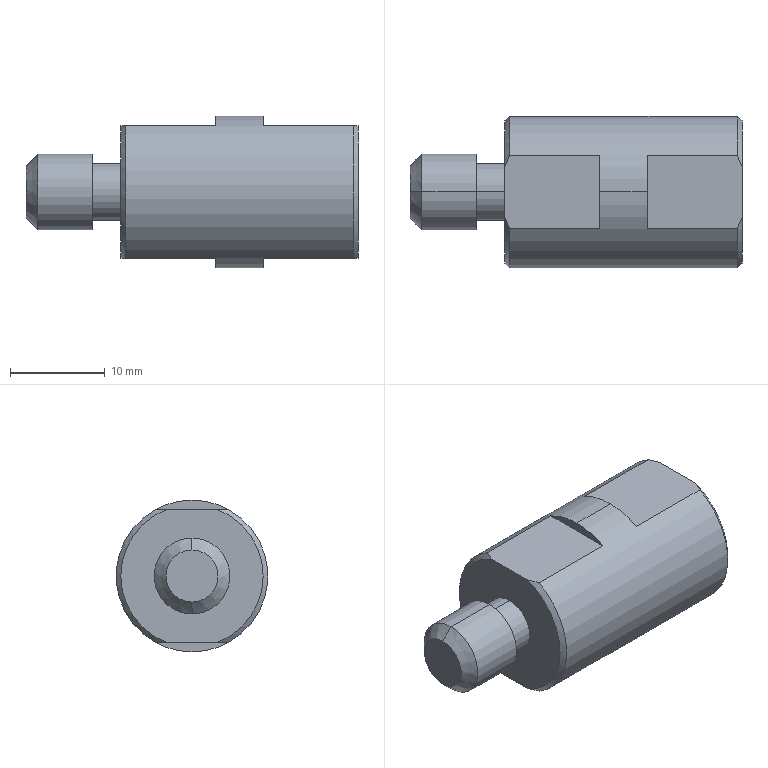Part | STEP file | PSSAGD16-27-F10-M8-N8-WSC0-X0-4 | 1 solid | 32 faces | box 35 x 16 x 16 mm | volume 4383 mm3 | plane 12 | cylinder 10 | cone 10 | commonest cylinder face diameters 8 x4 6 x2 6.647 x2 16 x2
STEP:
#1=CARTESIAN_POINT('',(4.919,0.,3.324));
#2=VERTEX_POINT('',#1);
#3=CARTESIAN_POINT('',(4.919,0.,-3.324));
#4=VERTEX_POINT('',#3);
#5=CARTESIAN_POINT('',(4.919,0.,0.));
#6=DIRECTION('',(1.,0.,0.));
#7=DIRECTION('',(0.,0.,-1.));
#8=AXIS2_PLACEMENT_3D('',#5,#6,#7);
#9=CIRCLE('',#8,3.324);
#10=EDGE_CURVE('',#2,#4,#9,.T.);
#11=ORIENTED_EDGE('',*,*,#10,.F.);
#12=CARTESIAN_POINT('',(16.591,0.,3.324));
#13=VERTEX_POINT('',#12);
#14=CARTESIAN_POINT('',(27.,0.,3.324));
#15=DIRECTION('',(1.,0.,0.));
#16=VECTOR('',#15,1000.);
#17=LINE('',#14,#16);
#18=EDGE_CURVE('',#2,#13,#17,.T.);
#19=ORIENTED_EDGE('',*,*,#18,.T.);
#20=CARTESIAN_POINT('',(16.591,0.,-3.323));
#21=VERTEX_POINT('',#20);
#22=CARTESIAN_POINT('',(16.591,0.,0.));
#23=DIRECTION('',(-1.,0.,0.));
#24=DIRECTION('',(0.,0.,-1.));
#25=AXIS2_PLACEMENT_3D('',#22,#23,#24);
#26=CIRCLE('',#25,3.324);
#27=EDGE_CURVE('',#21,#13,#26,.T.);
#28=ORIENTED_EDGE('',*,*,#27,.F.);
#29=CARTESIAN_POINT('',(27.,0.,-3.324));
#30=DIRECTION('',(1.,0.,0.));
#31=VECTOR('',#30,1000.);
#32=LINE('',#29,#31);
#33=EDGE_CURVE('',#4,#21,#32,.T.);
#34=ORIENTED_EDGE('',*,*,#33,.F.);
#35=EDGE_LOOP('',(#11,#19,#28,#34));
#36=FACE_OUTER_BOUND('',#35,.T.);
#37=CARTESIAN_POINT('',(27.,0.,0.));
#38=DIRECTION('',(1.,0.,0.));
#39=DIRECTION('',(0.,0.,-1.));
#40=AXIS2_PLACEMENT_3D('',#37,#38,#39);
#41=CYLINDRICAL_SURFACE('',#40,3.324);
#42=ADVANCED_FACE('',(#36),#41,.F.);
#43=CARTESIAN_POINT('',(3.,0.,0.));
#44=VERTEX_POINT('',#43);
#45=CARTESIAN_POINT('',(3.,0.,0.));
#46=DIRECTION('',(0.5,0.,-0.866));
#47=VECTOR('',#46,1000.);
#48=LINE('',#45,#47);
#49=EDGE_CURVE('',#44,#4,#48,.T.);
#50=ORIENTED_EDGE('',*,*,#49,.F.);
#51=CARTESIAN_POINT('',(3.,0.,0.));
#52=DIRECTION('',(0.5,0.,0.866));
#53=VECTOR('',#52,1000.);
#54=LINE('',#51,#53);
#55=EDGE_CURVE('',#44,#2,#54,.T.);
#56=ORIENTED_EDGE('',*,*,#55,.T.);
#57=ORIENTED_EDGE('',*,*,#10,.T.);
#58=EDGE_LOOP('',(#50,#56,#57));
#59=FACE_OUTER_BOUND('',#58,.T.);
#60=CARTESIAN_POINT('',(1003.,0.,0.));
#61=DIRECTION('',(1.,0.,0.));
#62=DIRECTION('',(0.,0.,-1.));
#63=AXIS2_PLACEMENT_3D('',#60,#61,#62);
#64=CONICAL_SURFACE('',#63,1732.051,1.047);
#65=ADVANCED_FACE('',(#59),#64,.F.);
#66=ORIENTED_EDGE('',*,*,#27,.T.);
#67=CARTESIAN_POINT('',(17.267,0.,4.));
#68=VERTEX_POINT('',#67);
#69=CARTESIAN_POINT('',(17.267,0.,4.));
#70=DIRECTION('',(0.7071,0.,0.7071));
#71=VECTOR('',#70,1000.);
#72=LINE('',#69,#71);
#73=EDGE_CURVE('',#13,#68,#72,.T.);
#74=ORIENTED_EDGE('',*,*,#73,.T.);
#75=CARTESIAN_POINT('',(17.267,0.,-4.));
#76=VERTEX_POINT('',#75);
#77=CARTESIAN_POINT('',(17.267,0.,0.));
#78=DIRECTION('',(-1.,0.,0.));
#79=DIRECTION('',(0.,0.,1.));
#80=AXIS2_PLACEMENT_3D('',#77,#78,#79);
#81=CIRCLE('',#80,4.);
#82=EDGE_CURVE('',#76,#68,#81,.T.);
#83=ORIENTED_EDGE('',*,*,#82,.F.);
#84=CARTESIAN_POINT('',(17.267,0.,-4.));
#85=DIRECTION('',(0.7071,0.,-0.7071));
#86=VECTOR('',#85,1000.);
#87=LINE('',#84,#86);
#88=EDGE_CURVE('',#21,#76,#87,.T.);
#89=ORIENTED_EDGE('',*,*,#88,.F.);
#90=EDGE_LOOP('',(#66,#74,#83,#89));
#91=FACE_OUTER_BOUND('',#90,.T.);
#92=CARTESIAN_POINT('',(17.267,0.,0.));
#93=DIRECTION('',(1.,0.,0.));
#94=DIRECTION('',(0.,0.,-1.));
#95=AXIS2_PLACEMENT_3D('',#92,#93,#94);
#96=CONICAL_SURFACE('',#95,4.,0.7854);
#97=ADVANCED_FACE('',(#91),#96,.F.);
#98=CARTESIAN_POINT('',(25.,0.,-4.));
#99=VERTEX_POINT('',#98);
#100=CARTESIAN_POINT('',(25.,0.,4.));
#101=VERTEX_POINT('',#100);
#102=CARTESIAN_POINT('',(25.,0.,0.));
#103=DIRECTION('',(-1.,0.,0.));
#104=DIRECTION('',(0.,0.,1.));
#105=AXIS2_PLACEMENT_3D('',#102,#103,#104);
#106=CIRCLE('',#105,4.);
#107=EDGE_CURVE('',#99,#101,#106,.T.);
#108=ORIENTED_EDGE('',*,*,#107,.F.);
#109=CARTESIAN_POINT('',(16.5,0.,-4.));
#110=DIRECTION('',(-1.,0.,0.));
#111=VECTOR('',#110,1000.);
#112=LINE('',#109,#111);
#113=EDGE_CURVE('',#99,#76,#112,.T.);
#114=ORIENTED_EDGE('',*,*,#113,.T.);
#115=ORIENTED_EDGE('',*,*,#82,.T.);
#116=CARTESIAN_POINT('',(16.5,0.,4.));
#117=DIRECTION('',(-1.,0.,0.));
#118=VECTOR('',#117,1000.);
#119=LINE('',#116,#118);
#120=EDGE_CURVE('',#101,#68,#119,.T.);
#121=ORIENTED_EDGE('',*,*,#120,.F.);
#122=EDGE_LOOP('',(#108,#114,#115,#121));
#123=FACE_OUTER_BOUND('',#122,.T.);
#124=CARTESIAN_POINT('',(16.5,0.,0.));
#125=DIRECTION('',(-1.,0.,0.));
#126=DIRECTION('',(0.,0.,1.));
#127=AXIS2_PLACEMENT_3D('',#124,#125,#126);
#128=CYLINDRICAL_SURFACE('',#127,4.);
#129=ADVANCED_FACE('',(#123),#128,.F.);
#130=CARTESIAN_POINT('',(-3.,0.,-3.));
#131=VERTEX_POINT('',#130);
#132=CARTESIAN_POINT('',(-3.,0.,3.));
#133=VERTEX_POINT('',#132);
#134=CARTESIAN_POINT('',(-3.,0.,0.));
#135=DIRECTION('',(1.,0.,0.));
#136=DIRECTION('',(0.,0.,-1.));
#137=AXIS2_PLACEMENT_3D('',#134,#135,#136);
#138=CIRCLE('',#137,3.);
#139=EDGE_CURVE('',#131,#133,#138,.T.);
#140=ORIENTED_EDGE('',*,*,#139,.T.);
#141=CARTESIAN_POINT('',(0.,0.,3.));
#142=VERTEX_POINT('',#141);
#143=CARTESIAN_POINT('',(27.,0.,3.));
#144=DIRECTION('',(1.,0.,0.));
#145=VECTOR('',#144,1000.);
#146=LINE('',#143,#145);
#147=EDGE_CURVE('',#133,#142,#146,.T.);
#148=ORIENTED_EDGE('',*,*,#147,.T.);
#149=CARTESIAN_POINT('',(0.,0.,-3.));
#150=VERTEX_POINT('',#149);
#151=CARTESIAN_POINT('',(0.,0.,0.));
#152=DIRECTION('',(1.,0.,0.));
#153=DIRECTION('',(0.,0.,-1.));
#154=AXIS2_PLACEMENT_3D('',#151,#152,#153);
#155=CIRCLE('',#154,3.);
#156=EDGE_CURVE('',#150,#142,#155,.T.);
#157=ORIENTED_EDGE('',*,*,#156,.F.);
#158=CARTESIAN_POINT('',(27.,0.,-3.));
#159=DIRECTION('',(1.,0.,0.));
#160=VECTOR('',#159,1000.);
#161=LINE('',#158,#160);
#162=EDGE_CURVE('',#131,#150,#161,.T.);
#163=ORIENTED_EDGE('',*,*,#162,.F.);
#164=EDGE_LOOP('',(#140,#148,#157,#163));
#165=FACE_OUTER_BOUND('',#164,.T.);
#166=CARTESIAN_POINT('',(27.,0.,0.));
#167=DIRECTION('',(1.,0.,0.));
#168=DIRECTION('',(0.,0.,-1.));
#169=AXIS2_PLACEMENT_3D('',#166,#167,#168);
#170=CYLINDRICAL_SURFACE('',#169,3.);
#171=ADVANCED_FACE('',(#165),#170,.T.);
#172=CARTESIAN_POINT('',(-8.75,0.,-4.));
#173=VERTEX_POINT('',#172);
#174=CARTESIAN_POINT('',(-8.75,0.,4.));
#175=VERTEX_POINT('',#174);
#176=CARTESIAN_POINT('',(-8.75,0.,0.));
#177=DIRECTION('',(1.,0.,0.));
#178=DIRECTION('',(0.,0.,-1.));
#179=AXIS2_PLACEMENT_3D('',#176,#177,#178);
#180=CIRCLE('',#179,4.);
#181=EDGE_CURVE('',#173,#175,#180,.T.);
#182=ORIENTED_EDGE('',*,*,#181,.T.);
#183=CARTESIAN_POINT('',(-3.,0.,4.));
#184=VERTEX_POINT('',#183);
#185=CARTESIAN_POINT('',(27.,0.,4.));
#186=DIRECTION('',(1.,0.,0.));
#187=VECTOR('',#186,1000.);
#188=LINE('',#185,#187);
#189=EDGE_CURVE('',#175,#184,#188,.T.);
#190=ORIENTED_EDGE('',*,*,#189,.T.);
#191=CARTESIAN_POINT('',(-3.,0.,-4.));
#192=VERTEX_POINT('',#191);
#193=CARTESIAN_POINT('',(-3.,0.,0.));
#194=DIRECTION('',(1.,0.,0.));
#195=DIRECTION('',(0.,0.,-1.));
#196=AXIS2_PLACEMENT_3D('',#193,#194,#195);
#197=CIRCLE('',#196,4.);
#198=EDGE_CURVE('',#192,#184,#197,.T.);
#199=ORIENTED_EDGE('',*,*,#198,.F.);
#200=CARTESIAN_POINT('',(27.,0.,-4.));
#201=DIRECTION('',(1.,0.,0.));
#202=VECTOR('',#201,1000.);
#203=LINE('',#200,#202);
#204=EDGE_CURVE('',#173,#192,#203,.T.);
#205=ORIENTED_EDGE('',*,*,#204,.F.);
#206=EDGE_LOOP('',(#182,#190,#199,#205));
#207=FACE_OUTER_BOUND('',#206,.T.);
#208=CARTESIAN_POINT('',(27.,0.,0.));
#209=DIRECTION('',(1.,0.,0.));
#210=DIRECTION('',(0.,0.,-1.));
#211=AXIS2_PLACEMENT_3D('',#208,#209,#210);
#212=CYLINDRICAL_SURFACE('',#211,4.);
#213=ADVANCED_FACE('',(#207),#212,.T.);
#214=CARTESIAN_POINT('',(-10.,0.,-2.75));
#215=VERTEX_POINT('',#214);
#216=CARTESIAN_POINT('',(-10.,0.,2.75));
#217=VERTEX_POINT('',#216);
#218=CARTESIAN_POINT('',(-10.,0.,0.));
#219=DIRECTION('',(1.,0.,0.));
#220=DIRECTION('',(0.,0.,-1.));
#221=AXIS2_PLACEMENT_3D('',#218,#219,#220);
#222=CIRCLE('',#221,2.75);
#223=EDGE_CURVE('',#215,#217,#222,.T.);
#224=ORIENTED_EDGE('',*,*,#223,.T.);
#225=CARTESIAN_POINT('',(-10.,0.,2.75));
#226=DIRECTION('',(0.7071,0.,0.7071));
#227=VECTOR('',#226,1000.);
#228=LINE('',#225,#227);
#229=EDGE_CURVE('',#217,#175,#228,.T.);
#230=ORIENTED_EDGE('',*,*,#229,.T.);
#231=ORIENTED_EDGE('',*,*,#181,.F.);
#232=CARTESIAN_POINT('',(-10.,0.,-2.75));
#233=DIRECTION('',(0.7071,0.,-0.7071));
#234=VECTOR('',#233,1000.);
#235=LINE('',#232,#234);
#236=EDGE_CURVE('',#215,#173,#235,.T.);
#237=ORIENTED_EDGE('',*,*,#236,.F.);
#238=EDGE_LOOP('',(#224,#230,#231,#237));
#239=FACE_OUTER_BOUND('',#238,.T.);
#240=CARTESIAN_POINT('',(-10.,0.,0.));
#241=DIRECTION('',(1.,0.,0.));
#242=DIRECTION('',(0.,0.,-1.));
#243=AXIS2_PLACEMENT_3D('',#240,#241,#242);
#244=CONICAL_SURFACE('',#243,2.75,0.7854);
#245=ADVANCED_FACE('',(#239),#244,.T.);
#246=CARTESIAN_POINT('',(10.,3.873,7.));
#247=VERTEX_POINT('',#246);
#248=CARTESIAN_POINT('',(10.,0.,8.));
#249=VERTEX_POINT('',#248);
#250=CARTESIAN_POINT('',(10.,0.,0.));
#251=DIRECTION('',(1.,0.,0.));
#252=DIRECTION('',(0.,0.,-1.));
#253=AXIS2_PLACEMENT_3D('',#250,#251,#252);
#254=CIRCLE('',#253,8.);
#255=EDGE_CURVE('',#247,#249,#254,.T.);
#256=ORIENTED_EDGE('',*,*,#255,.T.);
#257=CARTESIAN_POINT('',(15.,0.,8.));
#258=VERTEX_POINT('',#257);
#259=CARTESIAN_POINT('',(27.,0.,8.));
#260=DIRECTION('',(1.,0.,0.));
#261=VECTOR('',#260,1000.);
#262=LINE('',#259,#261);
#263=EDGE_CURVE('',#249,#258,#262,.T.);
#264=ORIENTED_EDGE('',*,*,#263,.T.);
#265=CARTESIAN_POINT('',(15.,3.873,7.));
#266=VERTEX_POINT('',#265);
#267=CARTESIAN_POINT('',(15.,0.,0.));
#268=DIRECTION('',(1.,0.,0.));
#269=DIRECTION('',(0.,0.,-1.));
#270=AXIS2_PLACEMENT_3D('',#267,#268,#269);
#271=CIRCLE('',#270,8.);
#272=EDGE_CURVE('',#266,#258,#271,.T.);
#273=ORIENTED_EDGE('',*,*,#272,.F.);
#274=CARTESIAN_POINT('',(24.5,3.873,7.));
#275=VERTEX_POINT('',#274);
#276=CARTESIAN_POINT('',(25.,3.873,7.));
#277=DIRECTION('',(-1.,0.,0.));
#278=VECTOR('',#277,1000.);
#279=LINE('',#276,#278);
#280=EDGE_CURVE('',#275,#266,#279,.T.);
#281=ORIENTED_EDGE('',*,*,#280,.F.);
#282=CARTESIAN_POINT('',(24.5,3.873,-7.));
#283=VERTEX_POINT('',#282);
#284=CARTESIAN_POINT('',(24.5,0.,0.));
#285=DIRECTION('',(1.,0.,0.));
#286=DIRECTION('',(0.,0.,-1.));
#287=AXIS2_PLACEMENT_3D('',#284,#285,#286);
#288=CIRCLE('',#287,8.);
#289=EDGE_CURVE('',#283,#275,#288,.T.);
#290=ORIENTED_EDGE('',*,*,#289,.F.);
#291=CARTESIAN_POINT('',(15.,3.873,-7.));
#292=VERTEX_POINT('',#291);
#293=CARTESIAN_POINT('',(25.,3.873,-7.));
#294=DIRECTION('',(1.,0.,0.));
#295=VECTOR('',#294,1000.);
#296=LINE('',#293,#295);
#297=EDGE_CURVE('',#292,#283,#296,.T.);
#298=ORIENTED_EDGE('',*,*,#297,.F.);
#299=CARTESIAN_POINT('',(15.,0.,-8.));
#300=VERTEX_POINT('',#299);
#301=CARTESIAN_POINT('',(15.,0.,0.));
#302=DIRECTION('',(1.,0.,0.));
#303=DIRECTION('',(0.,0.,-1.));
#304=AXIS2_PLACEMENT_3D('',#301,#302,#303);
#305=CIRCLE('',#304,8.);
#306=EDGE_CURVE('',#300,#292,#305,.T.);
#307=ORIENTED_EDGE('',*,*,#306,.F.);
#308=CARTESIAN_POINT('',(10.,0.,-8.));
#309=VERTEX_POINT('',#308);
#310=CARTESIAN_POINT('',(27.,0.,-8.));
#311=DIRECTION('',(1.,0.,0.));
#312=VECTOR('',#311,1000.);
#313=LINE('',#310,#312);
#314=EDGE_CURVE('',#309,#300,#313,.T.);
#315=ORIENTED_EDGE('',*,*,#314,.F.);
#316=CARTESIAN_POINT('',(10.,3.873,-7.));
#317=VERTEX_POINT('',#316);
#318=CARTESIAN_POINT('',(10.,0.,0.));
#319=DIRECTION('',(1.,0.,0.));
#320=DIRECTION('',(0.,0.,-1.));
#321=AXIS2_PLACEMENT_3D('',#318,#319,#320);
#322=CIRCLE('',#321,8.);
#323=EDGE_CURVE('',#309,#317,#322,.T.);
#324=ORIENTED_EDGE('',*,*,#323,.T.);
#325=CARTESIAN_POINT('',(0.5,3.873,-7.));
#326=VERTEX_POINT('',#325);
#327=CARTESIAN_POINT('',(27.,3.873,-7.));
#328=DIRECTION('',(-1.,0.,0.));
#329=VECTOR('',#328,1000.);
#330=LINE('',#327,#329);
#331=EDGE_CURVE('',#317,#326,#330,.T.);
#332=ORIENTED_EDGE('',*,*,#331,.T.);
#333=CARTESIAN_POINT('',(0.5,3.873,7.));
#334=VERTEX_POINT('',#333);
#335=CARTESIAN_POINT('',(0.5,0.,0.));
#336=DIRECTION('',(1.,0.,0.));
#337=DIRECTION('',(0.,0.,-1.));
#338=AXIS2_PLACEMENT_3D('',#335,#336,#337);
#339=CIRCLE('',#338,8.);
#340=EDGE_CURVE('',#326,#334,#339,.T.);
#341=ORIENTED_EDGE('',*,*,#340,.T.);
#342=CARTESIAN_POINT('',(27.,3.873,7.));
#343=DIRECTION('',(1.,0.,0.));
#344=VECTOR('',#343,1000.);
#345=LINE('',#342,#344);
#346=EDGE_CURVE('',#334,#247,#345,.T.);
#347=ORIENTED_EDGE('',*,*,#346,.T.);
#348=EDGE_LOOP('',(#256,#264,#273,#281,#290,#298,#307,#315,#324,#332,#341,#347));
#349=FACE_OUTER_BOUND('',#348,.T.);
#350=CARTESIAN_POINT('',(27.,0.,0.));
#351=DIRECTION('',(1.,0.,0.));
#352=DIRECTION('',(0.,0.,-1.));
#353=AXIS2_PLACEMENT_3D('',#350,#351,#352);
#354=CYLINDRICAL_SURFACE('',#353,8.);
#355=ADVANCED_FACE('',(#349),#354,.T.);
#356=ORIENTED_EDGE('',*,*,#263,.F.);
#357=CARTESIAN_POINT('',(10.,-3.873,7.));
#358=VERTEX_POINT('',#357);
#359=CARTESIAN_POINT('',(10.,0.,0.));
#360=DIRECTION('',(1.,0.,0.));
#361=DIRECTION('',(0.,0.,-1.));
#362=AXIS2_PLACEMENT_3D('',#359,#360,#361);
#363=CIRCLE('',#362,8.);
#364=EDGE_CURVE('',#249,#358,#363,.T.);
#365=ORIENTED_EDGE('',*,*,#364,.T.);
#366=CARTESIAN_POINT('',(0.5,-3.873,7.));
#367=VERTEX_POINT('',#366);
#368=CARTESIAN_POINT('',(27.,-3.873,7.));
#369=DIRECTION('',(-1.,0.,0.));
#370=VECTOR('',#369,1000.);
#371=LINE('',#368,#370);
#372=EDGE_CURVE('',#358,#367,#371,.T.);
#373=ORIENTED_EDGE('',*,*,#372,.T.);
#374=CARTESIAN_POINT('',(0.5,-3.873,-7.));
#375=VERTEX_POINT('',#374);
#376=CARTESIAN_POINT('',(0.5,0.,0.));
#377=DIRECTION('',(1.,0.,0.));
#378=DIRECTION('',(0.,0.,-1.));
#379=AXIS2_PLACEMENT_3D('',#376,#377,#378);
#380=CIRCLE('',#379,8.);
#381=EDGE_CURVE('',#367,#375,#380,.T.);
#382=ORIENTED_EDGE('',*,*,#381,.T.);
#383=CARTESIAN_POINT('',(10.,-3.873,-7.));
#384=VERTEX_POINT('',#383);
#385=CARTESIAN_POINT('',(27.,-3.873,-7.));
#386=DIRECTION('',(1.,0.,0.));
#387=VECTOR('',#386,1000.);
#388=LINE('',#385,#387);
#389=EDGE_CURVE('',#375,#384,#388,.T.);
#390=ORIENTED_EDGE('',*,*,#389,.T.);
#391=CARTESIAN_POINT('',(10.,0.,0.));
#392=DIRECTION('',(1.,0.,0.));
#393=DIRECTION('',(0.,0.,-1.));
#394=AXIS2_PLACEMENT_3D('',#391,#392,#393);
#395=CIRCLE('',#394,8.);
#396=EDGE_CURVE('',#384,#309,#395,.T.);
#397=ORIENTED_EDGE('',*,*,#396,.T.);
#398=ORIENTED_EDGE('',*,*,#314,.T.);
#399=CARTESIAN_POINT('',(15.,-3.873,-7.));
#400=VERTEX_POINT('',#399);
#401=CARTESIAN_POINT('',(15.,0.,0.));
#402=DIRECTION('',(1.,0.,0.));
#403=DIRECTION('',(0.,0.,-1.));
#404=AXIS2_PLACEMENT_3D('',#401,#402,#403);
#405=CIRCLE('',#404,8.);
#406=EDGE_CURVE('',#400,#300,#405,.T.);
#407=ORIENTED_EDGE('',*,*,#406,.F.);
#408=CARTESIAN_POINT('',(24.5,-3.873,-7.));
#409=VERTEX_POINT('',#408);
#410=CARTESIAN_POINT('',(25.,-3.873,-7.));
#411=DIRECTION('',(-1.,0.,0.));
#412=VECTOR('',#411,1000.);
#413=LINE('',#410,#412);
#414=EDGE_CURVE('',#409,#400,#413,.T.);
#415=ORIENTED_EDGE('',*,*,#414,.F.);
#416=CARTESIAN_POINT('',(24.5,-3.873,7.));
#417=VERTEX_POINT('',#416);
#418=CARTESIAN_POINT('',(24.5,0.,0.));
#419=DIRECTION('',(1.,0.,0.));
#420=DIRECTION('',(0.,0.,-1.));
#421=AXIS2_PLACEMENT_3D('',#418,#419,#420);
#422=CIRCLE('',#421,8.);
#423=EDGE_CURVE('',#417,#409,#422,.T.);
#424=ORIENTED_EDGE('',*,*,#423,.F.);
#425=CARTESIAN_POINT('',(15.,-3.873,7.));
#426=VERTEX_POINT('',#425);
#427=CARTESIAN_POINT('',(25.,-3.873,7.));
#428=DIRECTION('',(1.,0.,0.));
#429=VECTOR('',#428,1000.);
#430=LINE('',#427,#429);
#431=EDGE_CURVE('',#426,#417,#430,.T.);
#432=ORIENTED_EDGE('',*,*,#431,.F.);
#433=CARTESIAN_POINT('',(15.,0.,0.));
#434=DIRECTION('',(1.,0.,0.));
#435=DIRECTION('',(0.,0.,-1.));
#436=AXIS2_PLACEMENT_3D('',#433,#434,#435);
#437=CIRCLE('',#436,8.);
#438=EDGE_CURVE('',#258,#426,#437,.T.);
#439=ORIENTED_EDGE('',*,*,#438,.F.);
#440=EDGE_LOOP('',(#356,#365,#373,#382,#390,#397,#398,#407,#415,#424,#432,#439));
#441=FACE_OUTER_BOUND('',#440,.T.);
#442=CARTESIAN_POINT('',(27.,0.,0.));
#443=DIRECTION('',(1.,0.,0.));
#444=DIRECTION('',(0.,0.,-1.));
#445=AXIS2_PLACEMENT_3D('',#442,#443,#444);
#446=CYLINDRICAL_SURFACE('',#445,8.);
#447=ADVANCED_FACE('',(#441),#446,.T.);
#448=CARTESIAN_POINT('',(25.,-2.693,-7.));
#449=VERTEX_POINT('',#448);
#450=CARTESIAN_POINT('',(25.,-2.693,-7.));
#451=CARTESIAN_POINT('',(24.856,-3.095,-7.));
#452=CARTESIAN_POINT('',(24.687,-3.487,-7.));
#453=CARTESIAN_POINT('',(24.5,-3.873,-7.));
#454=B_SPLINE_CURVE_WITH_KNOTS('',3,(#450,#451,#452,#453),.UNSPECIFIED.,.F.,.F.,(4,4),(0.006725,0.007986),.UNSPECIFIED.);
#455=EDGE_CURVE('',#449,#409,#454,.T.);
#456=ORIENTED_EDGE('',*,*,#455,.F.);
#457=CARTESIAN_POINT('',(25.,-2.693,7.));
#458=VERTEX_POINT('',#457);
#459=CARTESIAN_POINT('',(25.,0.,0.));
#460=DIRECTION('',(1.,0.,0.));
#461=DIRECTION('',(0.,0.,-1.));
#462=AXIS2_PLACEMENT_3D('',#459,#460,#461);
#463=CIRCLE('',#462,7.5);
#464=EDGE_CURVE('',#458,#449,#463,.T.);
#465=ORIENTED_EDGE('',*,*,#464,.F.);
#466=CARTESIAN_POINT('',(24.5,-3.873,7.));
#467=CARTESIAN_POINT('',(24.688,-3.486,7.));
#468=CARTESIAN_POINT('',(24.856,-3.093,7.));
#469=CARTESIAN_POINT('',(25.,-2.693,7.));
#470=B_SPLINE_CURVE_WITH_KNOTS('',3,(#466,#467,#468,#469),.UNSPECIFIED.,.F.,.F.,(4,4),(0.000001583,0.001274),.UNSPECIFIED.);
#471=EDGE_CURVE('',#417,#458,#470,.T.);
#472=ORIENTED_EDGE('',*,*,#471,.F.);
#473=ORIENTED_EDGE('',*,*,#423,.T.);
#474=EDGE_LOOP('',(#456,#465,#472,#473));
#475=FACE_OUTER_BOUND('',#474,.T.);
#476=CARTESIAN_POINT('',(24.5,0.,0.));
#477=DIRECTION('',(-1.,0.,0.));
#478=DIRECTION('',(0.,0.,1.));
#479=AXIS2_PLACEMENT_3D('',#476,#477,#478);
#480=CONICAL_SURFACE('',#479,8.,0.7854);
#481=ADVANCED_FACE('',(#475),#480,.T.);
#482=CARTESIAN_POINT('',(25.,2.693,7.));
#483=VERTEX_POINT('',#482);
#484=CARTESIAN_POINT('',(25.,2.693,7.));
#485=CARTESIAN_POINT('',(24.856,3.095,7.));
#486=CARTESIAN_POINT('',(24.687,3.487,7.));
#487=CARTESIAN_POINT('',(24.5,3.873,7.));
#488=B_SPLINE_CURVE_WITH_KNOTS('',3,(#484,#485,#486,#487),.UNSPECIFIED.,.F.,.F.,(4,4),(0.006725,0.007986),.UNSPECIFIED.);
#489=EDGE_CURVE('',#483,#275,#488,.T.);
#490=ORIENTED_EDGE('',*,*,#489,.F.);
#491=CARTESIAN_POINT('',(25.,2.693,-7.));
#492=VERTEX_POINT('',#491);
#493=CARTESIAN_POINT('',(25.,0.,0.));
#494=DIRECTION('',(1.,0.,0.));
#495=DIRECTION('',(0.,0.,-1.));
#496=AXIS2_PLACEMENT_3D('',#493,#494,#495);
#497=CIRCLE('',#496,7.5);
#498=EDGE_CURVE('',#492,#483,#497,.T.);
#499=ORIENTED_EDGE('',*,*,#498,.F.);
#500=CARTESIAN_POINT('',(24.5,3.873,-7.));
#501=CARTESIAN_POINT('',(24.688,3.486,-7.));
#502=CARTESIAN_POINT('',(24.856,3.093,-7.));
#503=CARTESIAN_POINT('',(25.,2.693,-7.));
#504=B_SPLINE_CURVE_WITH_KNOTS('',3,(#500,#501,#502,#503),.UNSPECIFIED.,.F.,.F.,(4,4),(0.000001583,0.001274),.UNSPECIFIED.);
#505=EDGE_CURVE('',#283,#492,#504,.T.);
#506=ORIENTED_EDGE('',*,*,#505,.F.);
#507=ORIENTED_EDGE('',*,*,#289,.T.);
#508=EDGE_LOOP('',(#490,#499,#506,#507));
#509=FACE_OUTER_BOUND('',#508,.T.);
#510=CARTESIAN_POINT('',(24.5,0.,0.));
#511=DIRECTION('',(-1.,0.,0.));
#512=DIRECTION('',(0.,0.,1.));
#513=AXIS2_PLACEMENT_3D('',#510,#511,#512);
#514=CONICAL_SURFACE('',#513,8.,0.7854);
#515=ADVANCED_FACE('',(#509),#514,.T.);
#516=CARTESIAN_POINT('',(25.,0.,0.));
#517=DIRECTION('',(-1.,0.,0.));
#518=DIRECTION('',(0.,0.,1.));
#519=AXIS2_PLACEMENT_3D('',#516,#517,#518);
#520=CIRCLE('',#519,4.);
#521=EDGE_CURVE('',#101,#99,#520,.T.);
#522=ORIENTED_EDGE('',*,*,#521,.T.);
#523=ORIENTED_EDGE('',*,*,#107,.T.);
#524=EDGE_LOOP('',(#522,#523));
#525=FACE_BOUND('',#524,.T.);
#526=CARTESIAN_POINT('',(25.,7.5,-7.));
#527=DIRECTION('',(0.,-1.,0.));
#528=VECTOR('',#527,1000.);
#529=LINE('',#526,#528);
#530=EDGE_CURVE('',#492,#449,#529,.T.);
#531=ORIENTED_EDGE('',*,*,#530,.F.);
#532=ORIENTED_EDGE('',*,*,#498,.T.);
#533=CARTESIAN_POINT('',(25.,7.5,7.));
#534=DIRECTION('',(0.,1.,0.));
#535=VECTOR('',#534,1000.);
#536=LINE('',#533,#535);
#537=EDGE_CURVE('',#458,#483,#536,.T.);
#538=ORIENTED_EDGE('',*,*,#537,.F.);
#539=ORIENTED_EDGE('',*,*,#464,.T.);
#540=EDGE_LOOP('',(#531,#532,#538,#539));
#541=FACE_OUTER_BOUND('',#540,.T.);
#542=CARTESIAN_POINT('',(25.,7.5,0.));
#543=DIRECTION('',(-1.,0.,0.));
#544=DIRECTION('',(0.,0.,1.));
#545=AXIS2_PLACEMENT_3D('',#542,#543,#544);
#546=PLANE('',#545);
#547=ADVANCED_FACE('',(#525,#541),#546,.F.);
#548=CARTESIAN_POINT('',(0.,-2.693,7.));
#549=VERTEX_POINT('',#548);
#550=CARTESIAN_POINT('',(0.,-2.693,-7.));
#551=VERTEX_POINT('',#550);
#552=CARTESIAN_POINT('',(0.,0.,0.));
#553=DIRECTION('',(1.,0.,0.));
#554=DIRECTION('',(0.,0.,-1.));
#555=AXIS2_PLACEMENT_3D('',#552,#553,#554);
#556=CIRCLE('',#555,7.5);
#557=EDGE_CURVE('',#549,#551,#556,.T.);
#558=ORIENTED_EDGE('',*,*,#557,.T.);
#559=CARTESIAN_POINT('',(0.,-2.693,-7.));
#560=CARTESIAN_POINT('',(0.1444,-3.095,-7.));
#561=CARTESIAN_POINT('',(0.3133,-3.487,-7.));
#562=CARTESIAN_POINT('',(0.5,-3.873,-7.));
#563=B_SPLINE_CURVE_WITH_KNOTS('',3,(#559,#560,#561,#562),.UNSPECIFIED.,.F.,.F.,(4,4),(0.006725,0.007986),.UNSPECIFIED.);
#564=EDGE_CURVE('',#551,#375,#563,.T.);
#565=ORIENTED_EDGE('',*,*,#564,.T.);
#566=ORIENTED_EDGE('',*,*,#381,.F.);
#567=CARTESIAN_POINT('',(0.5,-3.873,7.));
#568=CARTESIAN_POINT('',(0.3124,-3.486,7.));
#569=CARTESIAN_POINT('',(0.1437,-3.093,7.));
#570=CARTESIAN_POINT('',(0.,-2.693,7.));
#571=B_SPLINE_CURVE_WITH_KNOTS('',3,(#567,#568,#569,#570),.UNSPECIFIED.,.F.,.F.,(4,4),(0.000001583,0.001274),.UNSPECIFIED.);
#572=EDGE_CURVE('',#367,#549,#571,.T.);
#573=ORIENTED_EDGE('',*,*,#572,.T.);
#574=EDGE_LOOP('',(#558,#565,#566,#573));
#575=FACE_OUTER_BOUND('',#574,.T.);
#576=CARTESIAN_POINT('',(0.,0.,0.));
#577=DIRECTION('',(1.,0.,0.));
#578=DIRECTION('',(0.,0.,-1.));
#579=AXIS2_PLACEMENT_3D('',#576,#577,#578);
#580=CONICAL_SURFACE('',#579,7.5,0.7854);
#581=ADVANCED_FACE('',(#575),#580,.T.);
#582=ORIENTED_EDGE('',*,*,#223,.F.);
#583=CARTESIAN_POINT('',(-10.,0.,0.));
#584=DIRECTION('',(1.,0.,0.));
#585=DIRECTION('',(0.,0.,-1.));
#586=AXIS2_PLACEMENT_3D('',#583,#584,#585);
#587=CIRCLE('',#586,2.75);
#588=EDGE_CURVE('',#217,#215,#587,.T.);
#589=ORIENTED_EDGE('',*,*,#588,.F.);
#590=EDGE_LOOP('',(#582,#589));
#591=FACE_OUTER_BOUND('',#590,.T.);
#592=CARTESIAN_POINT('',(-10.,0.,0.));
#593=DIRECTION('',(1.,0.,0.));
#594=DIRECTION('',(0.,0.,-1.));
#595=AXIS2_PLACEMENT_3D('',#592,#593,#594);
#596=PLANE('',#595);
#597=ADVANCED_FACE('',(#591),#596,.F.);
#598=ORIENTED_EDGE('',*,*,#229,.F.);
#599=ORIENTED_EDGE('',*,*,#588,.T.);
#600=ORIENTED_EDGE('',*,*,#236,.T.);
#601=CARTESIAN_POINT('',(-8.75,0.,0.));
#602=DIRECTION('',(1.,0.,0.));
#603=DIRECTION('',(0.,0.,-1.));
#604=AXIS2_PLACEMENT_3D('',#601,#602,#603);
#605=CIRCLE('',#604,4.);
#606=EDGE_CURVE('',#175,#173,#605,.T.);
#607=ORIENTED_EDGE('',*,*,#606,.F.);
#608=EDGE_LOOP('',(#598,#599,#600,#607));
#609=FACE_OUTER_BOUND('',#608,.T.);
#610=CARTESIAN_POINT('',(-10.,0.,0.));
#611=DIRECTION('',(1.,0.,0.));
#612=DIRECTION('',(0.,0.,-1.));
#613=AXIS2_PLACEMENT_3D('',#610,#611,#612);
#614=CONICAL_SURFACE('',#613,2.75,0.7854);
#615=ADVANCED_FACE('',(#609),#614,.T.);
#616=ORIENTED_EDGE('',*,*,#189,.F.);
#617=ORIENTED_EDGE('',*,*,#606,.T.);
#618=ORIENTED_EDGE('',*,*,#204,.T.);
#619=CARTESIAN_POINT('',(-3.,0.,0.));
#620=DIRECTION('',(1.,0.,0.));
#621=DIRECTION('',(0.,0.,-1.));
#622=AXIS2_PLACEMENT_3D('',#619,#620,#621);
#623=CIRCLE('',#622,4.);
#624=EDGE_CURVE('',#184,#192,#623,.T.);
#625=ORIENTED_EDGE('',*,*,#624,.F.);
#626=EDGE_LOOP('',(#616,#617,#618,#625));
#627=FACE_OUTER_BOUND('',#626,.T.);
#628=CARTESIAN_POINT('',(27.,0.,0.));
#629=DIRECTION('',(1.,0.,0.));
#630=DIRECTION('',(0.,0.,-1.));
#631=AXIS2_PLACEMENT_3D('',#628,#629,#630);
#632=CYLINDRICAL_SURFACE('',#631,4.);
#633=ADVANCED_FACE('',(#627),#632,.T.);
#634=ORIENTED_EDGE('',*,*,#139,.F.);
#635=CARTESIAN_POINT('',(-3.,0.,0.));
#636=DIRECTION('',(1.,0.,0.));
#637=DIRECTION('',(0.,0.,-1.));
#638=AXIS2_PLACEMENT_3D('',#635,#636,#637);
#639=CIRCLE('',#638,3.);
#640=EDGE_CURVE('',#133,#131,#639,.T.);
#641=ORIENTED_EDGE('',*,*,#640,.F.);
#642=EDGE_LOOP('',(#634,#641));
#643=FACE_BOUND('',#642,.T.);
#644=ORIENTED_EDGE('',*,*,#198,.T.);
#645=ORIENTED_EDGE('',*,*,#624,.T.);
#646=EDGE_LOOP('',(#644,#645));
#647=FACE_OUTER_BOUND('',#646,.T.);
#648=CARTESIAN_POINT('',(-3.,4.,0.));
#649=DIRECTION('',(-1.,0.,0.));
#650=DIRECTION('',(0.,0.,1.));
#651=AXIS2_PLACEMENT_3D('',#648,#649,#650);
#652=PLANE('',#651);
#653=ADVANCED_FACE('',(#643,#647),#652,.F.);
#654=ORIENTED_EDGE('',*,*,#147,.F.);
#655=ORIENTED_EDGE('',*,*,#640,.T.);
#656=ORIENTED_EDGE('',*,*,#162,.T.);
#657=CARTESIAN_POINT('',(0.,0.,0.));
#658=DIRECTION('',(1.,0.,0.));
#659=DIRECTION('',(0.,0.,-1.));
#660=AXIS2_PLACEMENT_3D('',#657,#658,#659);
#661=CIRCLE('',#660,3.);
#662=EDGE_CURVE('',#142,#150,#661,.T.);
#663=ORIENTED_EDGE('',*,*,#662,.F.);
#664=EDGE_LOOP('',(#654,#655,#656,#663));
#665=FACE_OUTER_BOUND('',#664,.T.);
#666=CARTESIAN_POINT('',(27.,0.,0.));
#667=DIRECTION('',(1.,0.,0.));
#668=DIRECTION('',(0.,0.,-1.));
#669=AXIS2_PLACEMENT_3D('',#666,#667,#668);
#670=CYLINDRICAL_SURFACE('',#669,3.);
#671=ADVANCED_FACE('',(#665),#670,.T.);
#672=CARTESIAN_POINT('',(0.,2.693,-7.));
#673=VERTEX_POINT('',#672);
#674=CARTESIAN_POINT('',(0.,2.693,7.));
#675=VERTEX_POINT('',#674);
#676=CARTESIAN_POINT('',(0.,0.,0.));
#677=DIRECTION('',(1.,0.,0.));
#678=DIRECTION('',(0.,0.,-1.));
#679=AXIS2_PLACEMENT_3D('',#676,#677,#678);
#680=CIRCLE('',#679,7.5);
#681=EDGE_CURVE('',#673,#675,#680,.T.);
#682=ORIENTED_EDGE('',*,*,#681,.F.);
#683=CARTESIAN_POINT('',(0.,-32.,-7.));
#684=DIRECTION('',(0.,1.,0.));
#685=VECTOR('',#684,1000.);
#686=LINE('',#683,#685);
#687=EDGE_CURVE('',#551,#673,#686,.T.);
#688=ORIENTED_EDGE('',*,*,#687,.F.);
#689=ORIENTED_EDGE('',*,*,#557,.F.);
#690=CARTESIAN_POINT('',(0.,32.,7.));
#691=DIRECTION('',(0.,-1.,0.));
#692=VECTOR('',#691,1000.);
#693=LINE('',#690,#692);
#694=EDGE_CURVE('',#675,#549,#693,.T.);
#695=ORIENTED_EDGE('',*,*,#694,.F.);
#696=EDGE_LOOP('',(#682,#688,#689,#695));
#697=FACE_OUTER_BOUND('',#696,.T.);
#698=ORIENTED_EDGE('',*,*,#156,.T.);
#699=ORIENTED_EDGE('',*,*,#662,.T.);
#700=EDGE_LOOP('',(#698,#699));
#701=FACE_BOUND('',#700,.T.);
#702=CARTESIAN_POINT('',(0.,3.,0.));
#703=DIRECTION('',(1.,0.,0.));
#704=DIRECTION('',(0.,0.,-1.));
#705=AXIS2_PLACEMENT_3D('',#702,#703,#704);
#706=PLANE('',#705);
#707=ADVANCED_FACE('',(#697,#701),#706,.F.);
#708=ORIENTED_EDGE('',*,*,#681,.T.);
#709=CARTESIAN_POINT('',(0.,2.693,7.));
#710=CARTESIAN_POINT('',(0.1444,3.095,7.));
#711=CARTESIAN_POINT('',(0.3133,3.487,7.));
#712=CARTESIAN_POINT('',(0.5,3.873,7.));
#713=B_SPLINE_CURVE_WITH_KNOTS('',3,(#709,#710,#711,#712),.UNSPECIFIED.,.F.,.F.,(4,4),(0.006725,0.007986),.UNSPECIFIED.);
#714=EDGE_CURVE('',#675,#334,#713,.T.);
#715=ORIENTED_EDGE('',*,*,#714,.T.);
#716=ORIENTED_EDGE('',*,*,#340,.F.);
#717=CARTESIAN_POINT('',(0.5,3.873,-7.));
#718=CARTESIAN_POINT('',(0.3124,3.486,-7.));
#719=CARTESIAN_POINT('',(0.1437,3.093,-7.));
#720=CARTESIAN_POINT('',(0.,2.693,-7.));
#721=B_SPLINE_CURVE_WITH_KNOTS('',3,(#717,#718,#719,#720),.UNSPECIFIED.,.F.,.F.,(4,4),(0.000001583,0.001274),.UNSPECIFIED.);
#722=EDGE_CURVE('',#326,#673,#721,.T.);
#723=ORIENTED_EDGE('',*,*,#722,.T.);
#724=EDGE_LOOP('',(#708,#715,#716,#723));
#725=FACE_OUTER_BOUND('',#724,.T.);
#726=CARTESIAN_POINT('',(0.,0.,0.));
#727=DIRECTION('',(1.,0.,0.));
#728=DIRECTION('',(0.,0.,-1.));
#729=AXIS2_PLACEMENT_3D('',#726,#727,#728);
#730=CONICAL_SURFACE('',#729,7.5,0.7854);
#731=ADVANCED_FACE('',(#725),#730,.T.);
#732=CARTESIAN_POINT('',(10.,-32.,-7.));
#733=DIRECTION('',(0.,1.,0.));
#734=VECTOR('',#733,1000.);
#735=LINE('',#732,#734);
#736=EDGE_CURVE('',#384,#317,#735,.T.);
#737=ORIENTED_EDGE('',*,*,#736,.T.);
#738=ORIENTED_EDGE('',*,*,#323,.F.);
#739=ORIENTED_EDGE('',*,*,#396,.F.);
#740=EDGE_LOOP('',(#737,#738,#739));
#741=FACE_OUTER_BOUND('',#740,.T.);
#742=CARTESIAN_POINT('',(10.,0.,0.));
#743=DIRECTION('',(1.,0.,0.));
#744=DIRECTION('',(0.,0.,-1.));
#745=AXIS2_PLACEMENT_3D('',#742,#743,#744);
#746=PLANE('',#745);
#747=ADVANCED_FACE('',(#741),#746,.F.);
#748=ORIENTED_EDGE('',*,*,#687,.T.);
#749=ORIENTED_EDGE('',*,*,#722,.F.);
#750=ORIENTED_EDGE('',*,*,#331,.F.);
#751=ORIENTED_EDGE('',*,*,#736,.F.);
#752=ORIENTED_EDGE('',*,*,#389,.F.);
#753=ORIENTED_EDGE('',*,*,#564,.F.);
#754=EDGE_LOOP('',(#748,#749,#750,#751,#752,#753));
#755=FACE_OUTER_BOUND('',#754,.T.);
#756=CARTESIAN_POINT('',(10.,-32.,-7.));
#757=DIRECTION('',(0.,0.,1.));
#758=DIRECTION('',(1.,0.,0.));
#759=AXIS2_PLACEMENT_3D('',#756,#757,#758);
#760=PLANE('',#759);
#761=ADVANCED_FACE('',(#755),#760,.F.);
#762=ORIENTED_EDGE('',*,*,#694,.T.);
#763=ORIENTED_EDGE('',*,*,#572,.F.);
#764=ORIENTED_EDGE('',*,*,#372,.F.);
#765=CARTESIAN_POINT('',(10.,32.,7.));
#766=DIRECTION('',(0.,-1.,0.));
#767=VECTOR('',#766,1000.);
#768=LINE('',#765,#767);
#769=EDGE_CURVE('',#247,#358,#768,.T.);
#770=ORIENTED_EDGE('',*,*,#769,.F.);
#771=ORIENTED_EDGE('',*,*,#346,.F.);
#772=ORIENTED_EDGE('',*,*,#714,.F.);
#773=EDGE_LOOP('',(#762,#763,#764,#770,#771,#772));
#774=FACE_OUTER_BOUND('',#773,.T.);
#775=CARTESIAN_POINT('',(10.,32.,7.));
#776=DIRECTION('',(0.,0.,-1.));
#777=DIRECTION('',(-1.,0.,0.));
#778=AXIS2_PLACEMENT_3D('',#775,#776,#777);
#779=PLANE('',#778);
#780=ADVANCED_FACE('',(#774),#779,.F.);
#781=ORIENTED_EDGE('',*,*,#769,.T.);
#782=ORIENTED_EDGE('',*,*,#364,.F.);
#783=ORIENTED_EDGE('',*,*,#255,.F.);
#784=EDGE_LOOP('',(#781,#782,#783));
#785=FACE_OUTER_BOUND('',#784,.T.);
#786=CARTESIAN_POINT('',(10.,0.,0.));
#787=DIRECTION('',(1.,0.,0.));
#788=DIRECTION('',(0.,0.,-1.));
#789=AXIS2_PLACEMENT_3D('',#786,#787,#788);
#790=PLANE('',#789);
#791=ADVANCED_FACE('',(#785),#790,.F.);
#792=ORIENTED_EDGE('',*,*,#431,.T.);
#793=ORIENTED_EDGE('',*,*,#471,.T.);
#794=ORIENTED_EDGE('',*,*,#537,.T.);
#795=ORIENTED_EDGE('',*,*,#489,.T.);
#796=ORIENTED_EDGE('',*,*,#280,.T.);
#797=CARTESIAN_POINT('',(15.,32.,7.));
#798=DIRECTION('',(0.,-1.,0.));
#799=VECTOR('',#798,1000.);
#800=LINE('',#797,#799);
#801=EDGE_CURVE('',#266,#426,#800,.T.);
#802=ORIENTED_EDGE('',*,*,#801,.T.);
#803=EDGE_LOOP('',(#792,#793,#794,#795,#796,#802));
#804=FACE_OUTER_BOUND('',#803,.T.);
#805=CARTESIAN_POINT('',(15.,32.,7.));
#806=DIRECTION('',(0.,0.,1.));
#807=DIRECTION('',(1.,0.,0.));
#808=AXIS2_PLACEMENT_3D('',#805,#806,#807);
#809=PLANE('',#808);
#810=ADVANCED_FACE('',(#804),#809,.T.);
#811=ORIENTED_EDGE('',*,*,#272,.T.);
#812=ORIENTED_EDGE('',*,*,#438,.T.);
#813=ORIENTED_EDGE('',*,*,#801,.F.);
#814=EDGE_LOOP('',(#811,#812,#813));
#815=FACE_OUTER_BOUND('',#814,.T.);
#816=CARTESIAN_POINT('',(15.,0.,0.));
#817=DIRECTION('',(1.,0.,0.));
#818=DIRECTION('',(0.,0.,-1.));
#819=AXIS2_PLACEMENT_3D('',#816,#817,#818);
#820=PLANE('',#819);
#821=ADVANCED_FACE('',(#815),#820,.T.);
#822=ORIENTED_EDGE('',*,*,#406,.T.);
#823=ORIENTED_EDGE('',*,*,#306,.T.);
#824=CARTESIAN_POINT('',(15.,-32.,-7.));
#825=DIRECTION('',(0.,1.,0.));
#826=VECTOR('',#825,1000.);
#827=LINE('',#824,#826);
#828=EDGE_CURVE('',#400,#292,#827,.T.);
#829=ORIENTED_EDGE('',*,*,#828,.F.);
#830=EDGE_LOOP('',(#822,#823,#829));
#831=FACE_OUTER_BOUND('',#830,.T.);
#832=CARTESIAN_POINT('',(15.,0.,0.));
#833=DIRECTION('',(1.,0.,0.));
#834=DIRECTION('',(0.,0.,-1.));
#835=AXIS2_PLACEMENT_3D('',#832,#833,#834);
#836=PLANE('',#835);
#837=ADVANCED_FACE('',(#831),#836,.T.);
#838=ORIENTED_EDGE('',*,*,#297,.T.);
#839=ORIENTED_EDGE('',*,*,#505,.T.);
#840=ORIENTED_EDGE('',*,*,#530,.T.);
#841=ORIENTED_EDGE('',*,*,#455,.T.);
#842=ORIENTED_EDGE('',*,*,#414,.T.);
#843=ORIENTED_EDGE('',*,*,#828,.T.);
#844=EDGE_LOOP('',(#838,#839,#840,#841,#842,#843));
#845=FACE_OUTER_BOUND('',#844,.T.);
#846=CARTESIAN_POINT('',(15.,-32.,-7.));
#847=DIRECTION('',(0.,0.,-1.));
#848=DIRECTION('',(-1.,0.,0.));
#849=AXIS2_PLACEMENT_3D('',#846,#847,#848);
#850=PLANE('',#849);
#851=ADVANCED_FACE('',(#845),#850,.T.);
#852=ORIENTED_EDGE('',*,*,#113,.F.);
#853=ORIENTED_EDGE('',*,*,#521,.F.);
#854=ORIENTED_EDGE('',*,*,#120,.T.);
#855=CARTESIAN_POINT('',(17.267,0.,0.));
#856=DIRECTION('',(-1.,0.,0.));
#857=DIRECTION('',(0.,0.,1.));
#858=AXIS2_PLACEMENT_3D('',#855,#856,#857);
#859=CIRCLE('',#858,4.);
#860=EDGE_CURVE('',#68,#76,#859,.T.);
#861=ORIENTED_EDGE('',*,*,#860,.T.);
#862=EDGE_LOOP('',(#852,#853,#854,#861));
#863=FACE_OUTER_BOUND('',#862,.T.);
#864=CARTESIAN_POINT('',(16.5,0.,0.));
#865=DIRECTION('',(-1.,0.,0.));
#866=DIRECTION('',(0.,0.,1.));
#867=AXIS2_PLACEMENT_3D('',#864,#865,#866);
#868=CYLINDRICAL_SURFACE('',#867,4.);
#869=ADVANCED_FACE('',(#863),#868,.F.);
#870=ORIENTED_EDGE('',*,*,#73,.F.);
#871=CARTESIAN_POINT('',(16.591,0.,0.));
#872=DIRECTION('',(-1.,0.,0.));
#873=DIRECTION('',(0.,0.,-1.));
#874=AXIS2_PLACEMENT_3D('',#871,#872,#873);
#875=CIRCLE('',#874,3.324);
#876=EDGE_CURVE('',#13,#21,#875,.T.);
#877=ORIENTED_EDGE('',*,*,#876,.T.);
#878=ORIENTED_EDGE('',*,*,#88,.T.);
#879=ORIENTED_EDGE('',*,*,#860,.F.);
#880=EDGE_LOOP('',(#870,#877,#878,#879));
#881=FACE_OUTER_BOUND('',#880,.T.);
#882=CARTESIAN_POINT('',(17.267,0.,0.));
#883=DIRECTION('',(1.,0.,0.));
#884=DIRECTION('',(0.,0.,-1.));
#885=AXIS2_PLACEMENT_3D('',#882,#883,#884);
#886=CONICAL_SURFACE('',#885,4.,0.7854);
#887=ADVANCED_FACE('',(#881),#886,.F.);
#888=ORIENTED_EDGE('',*,*,#55,.F.);
#889=ORIENTED_EDGE('',*,*,#49,.T.);
#890=CARTESIAN_POINT('',(4.919,0.,0.));
#891=DIRECTION('',(1.,0.,0.));
#892=DIRECTION('',(0.,0.,-1.));
#893=AXIS2_PLACEMENT_3D('',#890,#891,#892);
#894=CIRCLE('',#893,3.324);
#895=EDGE_CURVE('',#4,#2,#894,.T.);
#896=ORIENTED_EDGE('',*,*,#895,.T.);
#897=EDGE_LOOP('',(#888,#889,#896));
#898=FACE_OUTER_BOUND('',#897,.T.);
#899=CARTESIAN_POINT('',(1003.,0.,0.));
#900=DIRECTION('',(1.,0.,0.));
#901=DIRECTION('',(0.,0.,-1.));
#902=AXIS2_PLACEMENT_3D('',#899,#900,#901);
#903=CONICAL_SURFACE('',#902,1732.051,1.047);
#904=ADVANCED_FACE('',(#898),#903,.F.);
#905=ORIENTED_EDGE('',*,*,#18,.F.);
#906=ORIENTED_EDGE('',*,*,#895,.F.);
#907=ORIENTED_EDGE('',*,*,#33,.T.);
#908=ORIENTED_EDGE('',*,*,#876,.F.);
#909=EDGE_LOOP('',(#905,#906,#907,#908));
#910=FACE_OUTER_BOUND('',#909,.T.);
#911=CARTESIAN_POINT('',(27.,0.,0.));
#912=DIRECTION('',(1.,0.,0.));
#913=DIRECTION('',(0.,0.,-1.));
#914=AXIS2_PLACEMENT_3D('',#911,#912,#913);
#915=CYLINDRICAL_SURFACE('',#914,3.324);
#916=ADVANCED_FACE('',(#910),#915,.F.);
#917=CLOSED_SHELL('',(#42,#65,#97,#129,#171,#213,#245,#355,#447,#481,#515,#547,#581,#597,#615,#633,#653,#671,#707,#731,#747,#761,#780,#791,#810,#821,#837,#851,#869,#887,#904,#916));
#918=MANIFOLD_SOLID_BREP('',#917);
#919=CARTESIAN_POINT('',(0.,0.,0.));
#920=DIRECTION('',(0.,0.,1.));
#921=DIRECTION('',(1.,0.,0.));
#922=AXIS2_PLACEMENT_3D('',#919,#920,#921);
#923=(LENGTH_UNIT()NAMED_UNIT(*)SI_UNIT(.MILLI.,.METRE.));
#924=UNCERTAINTY_MEASURE_WITH_UNIT(LENGTH_MEASURE(0.00001),#923,'','');
#925=(NAMED_UNIT(*)PLANE_ANGLE_UNIT()SI_UNIT($,.RADIAN.));
#926=(NAMED_UNIT(*)SI_UNIT($,.STERADIAN.)SOLID_ANGLE_UNIT());
#927=(GEOMETRIC_REPRESENTATION_CONTEXT(3)GLOBAL_UNCERTAINTY_ASSIGNED_CONTEXT((#924))GLOBAL_UNIT_ASSIGNED_CONTEXT((#923,#925,#926))REPRESENTATION_CONTEXT('',''));
#928=ADVANCED_BREP_SHAPE_REPRESENTATION('',(#918,#922),#927);